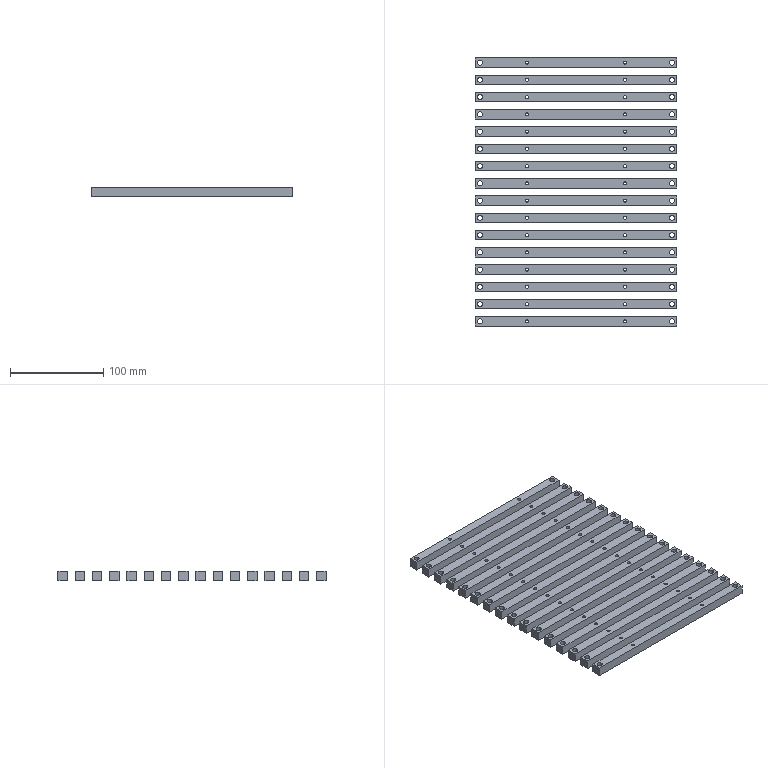CAM job | NX | 3-axis milling, drilling | part box 216 x 287.5 x 10 mm | stock box 220 x 291.5 x 11 mm
Tools:
number,name,description,diameter,corner_radius,flute_length,length,flutes
1,D63,Milling Tool-5 Parameters,63.0,0.0,50.0,75.0,2
7,D6A45,Milling Tool-5 Parameters,6.0,0.0,3.0,3.0,2
13,3.3ZT,Drilling Tool,3.3,0.0,35.0,50.0,2
17,M4,Milling Tool-5 Parameters,3.3,0.0,30.0,30.0,4
12,5.5ZT,Drilling Tool,5.5,0.0,35.0,50.0,2
6,D6,Milling Tool-5 Parameters,6.0,0.0,50.0,75.0,2
Operations:
program,operation,operation_type,tool,method,geometry_group,spindle_rpm,surface_speed,feed_per_tooth,feed_cut,feed_plunge,cut_length_mm,path_length_mm,cut_time_min,machine_time_min
1-292-219-10毛胚-AB胶,FLOOR_WALL,VolumeBased25DMillingOperation,D63,METHOD,A,6500.0,1286.0,0.0962,1250.0,100.0,3042.797,3096.797,2.434,2.44
1-292-219-10毛胚-AB胶,DRILLING_COPY_1,Operation,D6A45,METHOD,A,3000.0,56.0,0.0333,200.0,0.0,326.4,2232.521,1.632,1.823
1-292-219-10毛胚-AB胶,DRILLING_COPY_1_COPY_COPY_COPY_COPY_COPY,Operation,3.3ZT,METHOD,A,2000.0,20.0,0.0375,150.0,0.0,495.725,1811.744,3.305,3.436
1-292-219-10毛胚-AB胶,DRILLING_COPY_1_COPY_COPY_COPY_COPY_COPY_COPY_1,Operation,M4,METHOD,A,200.0,2.0,0.175,140.0,0.0,432.0,1684.293,3.086,3.211
1-292-219-10毛胚-AB胶,DRILLING_COPY_1_COPY_COPY_1_COPY_1,Operation,5.5ZT,METHOD,A,2000.0,18.0,0.03,120.0,0.0,484.876,1891.023,4.041,4.181
1-292-219-10毛胚-AB胶,ZLEVEL_PROFILE,ZLevelMilling,D6,METHOD,A,7000.0,219.0,0.2143,3000.0,1000.0,182010.094,184073.373,61.056,61.262
1-292-219-10毛胚-AB胶,ZLEVEL_PROFILE_COPY_1_COPY_COPY_COPY_COPY_2_COPY,ZLevelMilling,D6A45,METHOD,A,7000.0,131.0,0.0714,1000.0,1000.0,8032.583,23753.756,8.033,9.605
1-292-219-10毛胚-AB胶,ZLEVEL_PROFILE_COPY_1_1,ZLevelMilling,D6,METHOD,A,7000.0,219.0,0.0714,1000.0,1000.0,23245.721,27177.079,23.246,23.639